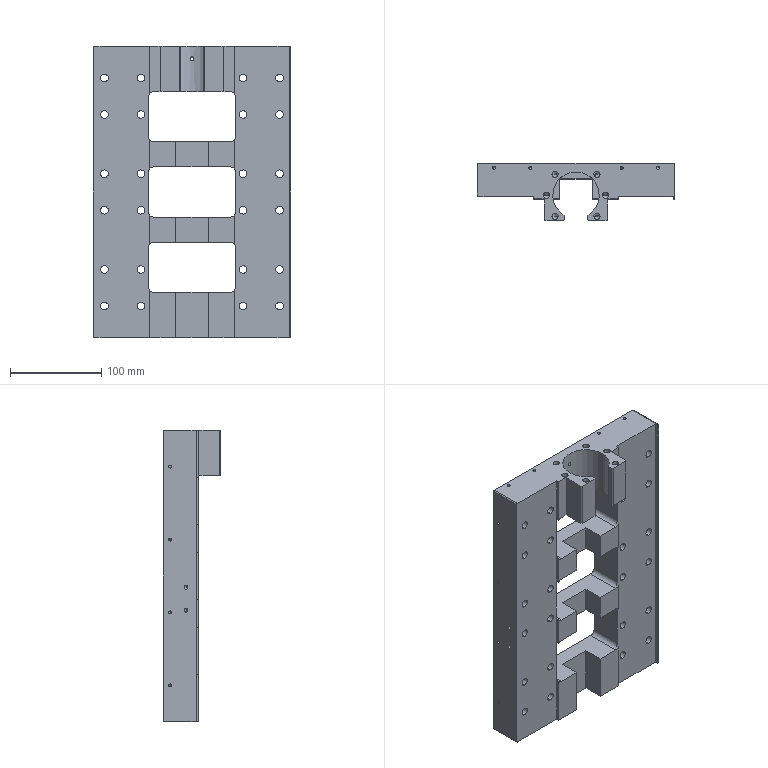Part | STEP file | 1 solid | 378 faces | box 217 x 63 x 320 mm | volume 1789943 mm3 | cylinder 214 | cone 84 | plane 80 | commonest cylinder face diameters 8.4 x48 15 x48 4.2 x40 3.3 x32 4 x12 6.8 x12